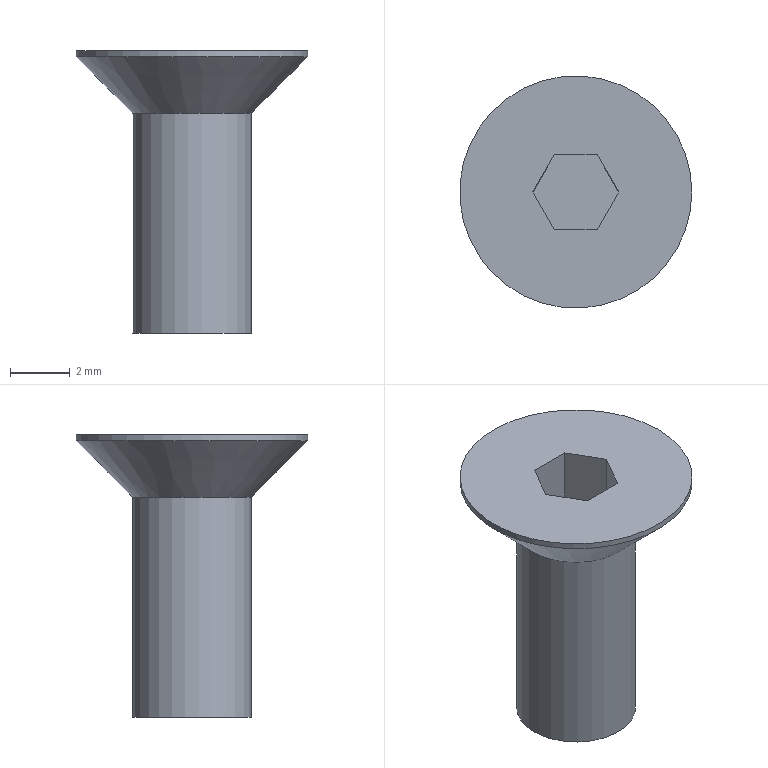Part | STEP file | Tube feed_id378_x_t | 1 solid | 12 faces | box 7.8 x 7.8 x 9.5 mm | volume 142 mm3 | plane 9 | cylinder 2 | cone 1 | commonest cylinder face diameters 4 x1 7.8 x1
STEP:
#1=CARTESIAN_POINT('',(0.,0.,0.));
#2=DIRECTION('',(0.,0.,1.));
#3=DIRECTION('',(1.,0.,0.));
#4=AXIS2_PLACEMENT_3D('',#1,#2,#3);
#5=CARTESIAN_POINT('',(351.278,11.286,-1.5));
#6=VERTEX_POINT('',#5);
#7=CARTESIAN_POINT('',(350.557,10.036,-1.5));
#8=VERTEX_POINT('',#7);
#9=CARTESIAN_POINT('',(351.278,11.286,-1.5));
#10=DIRECTION('',(-0.5,-0.866,0.));
#11=VECTOR('',#10,1.);
#12=LINE('',#9,#11);
#13=CARTESIAN_POINT('',(352.,10.036,-1.5));
#14=DIRECTION('',(0.,0.,1.));
#15=DIRECTION('',(1.,0.,0.));
#16=AXIS2_PLACEMENT_3D('',#13,#14,#15);
#17=PLANE('',#16);
#18=CARTESIAN_POINT('',(-0.7217,1.25));
#19=DIRECTION('',(-0.5,-0.866));
#20=VECTOR('',#19,1.);
#21=LINE('',#18,#20);
#22=(GEOMETRIC_REPRESENTATION_CONTEXT(2)PARAMETRIC_REPRESENTATION_CONTEXT()REPRESENTATION_CONTEXT('',''));
#23=DEFINITIONAL_REPRESENTATION('',(#21),#22);
#24=PCURVE('',#17,#23);
#25=CARTESIAN_POINT('',(351.278,11.286,-4.14));
#26=DIRECTION('',(-0.866,0.5,0.));
#27=DIRECTION('',(-0.5,-0.866,0.));
#28=AXIS2_PLACEMENT_3D('',#25,#26,#27);
#29=PLANE('',#28);
#30=CARTESIAN_POINT('',(0.,2.64));
#31=DIRECTION('',(1.,0.));
#32=VECTOR('',#31,1.);
#33=LINE('',#30,#32);
#34=(GEOMETRIC_REPRESENTATION_CONTEXT(2)PARAMETRIC_REPRESENTATION_CONTEXT()REPRESENTATION_CONTEXT('',''));
#35=DEFINITIONAL_REPRESENTATION('',(#33),#34);
#36=PCURVE('',#29,#35);
#37=SURFACE_CURVE('',#12,(#24,#36),.PCURVE_S1.);
#38=EDGE_CURVE('',#6,#8,#37,.T.);
#39=ORIENTED_EDGE('',*,*,#38,.F.);
#40=CARTESIAN_POINT('',(352.722,11.286,-1.5));
#41=VERTEX_POINT('',#40);
#42=CARTESIAN_POINT('',(352.722,11.286,-1.5));
#43=DIRECTION('',(-1.,0.,0.));
#44=VECTOR('',#43,1.);
#45=LINE('',#42,#44);
#46=CARTESIAN_POINT('',(0.7217,1.25));
#47=DIRECTION('',(-1.,0.));
#48=VECTOR('',#47,1.);
#49=LINE('',#46,#48);
#50=(GEOMETRIC_REPRESENTATION_CONTEXT(2)PARAMETRIC_REPRESENTATION_CONTEXT()REPRESENTATION_CONTEXT('',''));
#51=DEFINITIONAL_REPRESENTATION('',(#49),#50);
#52=PCURVE('',#17,#51);
#53=CARTESIAN_POINT('',(352.722,11.286,-4.14));
#54=DIRECTION('',(0.,1.,0.));
#55=DIRECTION('',(-1.,0.,0.));
#56=AXIS2_PLACEMENT_3D('',#53,#54,#55);
#57=PLANE('',#56);
#58=CARTESIAN_POINT('',(0.,2.64));
#59=DIRECTION('',(1.,0.));
#60=VECTOR('',#59,1.);
#61=LINE('',#58,#60);
#62=(GEOMETRIC_REPRESENTATION_CONTEXT(2)PARAMETRIC_REPRESENTATION_CONTEXT()REPRESENTATION_CONTEXT('',''));
#63=DEFINITIONAL_REPRESENTATION('',(#61),#62);
#64=PCURVE('',#57,#63);
#65=SURFACE_CURVE('',#45,(#52,#64),.PCURVE_S1.);
#66=EDGE_CURVE('',#41,#6,#65,.T.);
#67=ORIENTED_EDGE('',*,*,#66,.F.);
#68=CARTESIAN_POINT('',(353.443,10.036,-1.5));
#69=VERTEX_POINT('',#68);
#70=CARTESIAN_POINT('',(353.443,10.036,-1.5));
#71=DIRECTION('',(-0.5,0.866,0.));
#72=VECTOR('',#71,1.);
#73=LINE('',#70,#72);
#74=CARTESIAN_POINT('',(1.443,0.));
#75=DIRECTION('',(-0.5,0.866));
#76=VECTOR('',#75,1.);
#77=LINE('',#74,#76);
#78=(GEOMETRIC_REPRESENTATION_CONTEXT(2)PARAMETRIC_REPRESENTATION_CONTEXT()REPRESENTATION_CONTEXT('',''));
#79=DEFINITIONAL_REPRESENTATION('',(#77),#78);
#80=PCURVE('',#17,#79);
#81=CARTESIAN_POINT('',(353.443,10.036,-4.14));
#82=DIRECTION('',(0.866,0.5,0.));
#83=DIRECTION('',(-0.5,0.866,0.));
#84=AXIS2_PLACEMENT_3D('',#81,#82,#83);
#85=PLANE('',#84);
#86=CARTESIAN_POINT('',(0.,2.64));
#87=DIRECTION('',(1.,0.));
#88=VECTOR('',#87,1.);
#89=LINE('',#86,#88);
#90=(GEOMETRIC_REPRESENTATION_CONTEXT(2)PARAMETRIC_REPRESENTATION_CONTEXT()REPRESENTATION_CONTEXT('',''));
#91=DEFINITIONAL_REPRESENTATION('',(#89),#90);
#92=PCURVE('',#85,#91);
#93=SURFACE_CURVE('',#73,(#80,#92),.PCURVE_S1.);
#94=EDGE_CURVE('',#69,#41,#93,.T.);
#95=ORIENTED_EDGE('',*,*,#94,.F.);
#96=CARTESIAN_POINT('',(352.722,8.786,-1.5));
#97=VERTEX_POINT('',#96);
#98=CARTESIAN_POINT('',(352.722,8.786,-1.5));
#99=DIRECTION('',(0.5,0.866,0.));
#100=VECTOR('',#99,1.);
#101=LINE('',#98,#100);
#102=CARTESIAN_POINT('',(0.7217,-1.25));
#103=DIRECTION('',(0.5,0.866));
#104=VECTOR('',#103,1.);
#105=LINE('',#102,#104);
#106=(GEOMETRIC_REPRESENTATION_CONTEXT(2)PARAMETRIC_REPRESENTATION_CONTEXT()REPRESENTATION_CONTEXT('',''));
#107=DEFINITIONAL_REPRESENTATION('',(#105),#106);
#108=PCURVE('',#17,#107);
#109=CARTESIAN_POINT('',(352.722,8.786,-4.14));
#110=DIRECTION('',(0.866,-0.5,0.));
#111=DIRECTION('',(0.5,0.866,0.));
#112=AXIS2_PLACEMENT_3D('',#109,#110,#111);
#113=PLANE('',#112);
#114=CARTESIAN_POINT('',(0.,2.64));
#115=DIRECTION('',(1.,0.));
#116=VECTOR('',#115,1.);
#117=LINE('',#114,#116);
#118=(GEOMETRIC_REPRESENTATION_CONTEXT(2)PARAMETRIC_REPRESENTATION_CONTEXT()REPRESENTATION_CONTEXT('',''));
#119=DEFINITIONAL_REPRESENTATION('',(#117),#118);
#120=PCURVE('',#113,#119);
#121=SURFACE_CURVE('',#101,(#108,#120),.PCURVE_S1.);
#122=EDGE_CURVE('',#97,#69,#121,.T.);
#123=ORIENTED_EDGE('',*,*,#122,.F.);
#124=CARTESIAN_POINT('',(351.278,8.786,-1.5));
#125=VERTEX_POINT('',#124);
#126=CARTESIAN_POINT('',(351.278,8.786,-1.5));
#127=DIRECTION('',(1.,0.,0.));
#128=VECTOR('',#127,1.);
#129=LINE('',#126,#128);
#130=CARTESIAN_POINT('',(-0.7217,-1.25));
#131=DIRECTION('',(1.,0.));
#132=VECTOR('',#131,1.);
#133=LINE('',#130,#132);
#134=(GEOMETRIC_REPRESENTATION_CONTEXT(2)PARAMETRIC_REPRESENTATION_CONTEXT()REPRESENTATION_CONTEXT('',''));
#135=DEFINITIONAL_REPRESENTATION('',(#133),#134);
#136=PCURVE('',#17,#135);
#137=CARTESIAN_POINT('',(351.278,8.786,-4.14));
#138=DIRECTION('',(0.,-1.,0.));
#139=DIRECTION('',(1.,0.,0.));
#140=AXIS2_PLACEMENT_3D('',#137,#138,#139);
#141=PLANE('',#140);
#142=CARTESIAN_POINT('',(0.,2.64));
#143=DIRECTION('',(1.,0.));
#144=VECTOR('',#143,1.);
#145=LINE('',#142,#144);
#146=(GEOMETRIC_REPRESENTATION_CONTEXT(2)PARAMETRIC_REPRESENTATION_CONTEXT()REPRESENTATION_CONTEXT('',''));
#147=DEFINITIONAL_REPRESENTATION('',(#145),#146);
#148=PCURVE('',#141,#147);
#149=SURFACE_CURVE('',#129,(#136,#148),.PCURVE_S1.);
#150=EDGE_CURVE('',#125,#97,#149,.T.);
#151=ORIENTED_EDGE('',*,*,#150,.F.);
#152=CARTESIAN_POINT('',(350.557,10.036,-1.5));
#153=DIRECTION('',(0.5,-0.866,0.));
#154=VECTOR('',#153,1.);
#155=LINE('',#152,#154);
#156=CARTESIAN_POINT('',(-1.443,0.));
#157=DIRECTION('',(0.5,-0.866));
#158=VECTOR('',#157,1.);
#159=LINE('',#156,#158);
#160=(GEOMETRIC_REPRESENTATION_CONTEXT(2)PARAMETRIC_REPRESENTATION_CONTEXT()REPRESENTATION_CONTEXT('',''));
#161=DEFINITIONAL_REPRESENTATION('',(#159),#160);
#162=PCURVE('',#17,#161);
#163=CARTESIAN_POINT('',(350.557,10.036,-4.14));
#164=DIRECTION('',(-0.866,-0.5,0.));
#165=DIRECTION('',(0.5,-0.866,0.));
#166=AXIS2_PLACEMENT_3D('',#163,#164,#165);
#167=PLANE('',#166);
#168=CARTESIAN_POINT('',(0.,2.64));
#169=DIRECTION('',(1.,0.));
#170=VECTOR('',#169,1.);
#171=LINE('',#168,#170);
#172=(GEOMETRIC_REPRESENTATION_CONTEXT(2)PARAMETRIC_REPRESENTATION_CONTEXT()REPRESENTATION_CONTEXT('',''));
#173=DEFINITIONAL_REPRESENTATION('',(#171),#172);
#174=PCURVE('',#167,#173);
#175=SURFACE_CURVE('',#155,(#162,#174),.PCURVE_S1.);
#176=EDGE_CURVE('',#8,#125,#175,.T.);
#177=ORIENTED_EDGE('',*,*,#176,.F.);
#178=EDGE_LOOP('',(#39,#67,#95,#123,#151,#177));
#179=FACE_BOUND('',#178,.T.);
#180=CARTESIAN_POINT('',(355.9,10.036,-1.5));
#181=VERTEX_POINT('',#180);
#182=CARTESIAN_POINT('',(352.,10.036,-1.5));
#183=DIRECTION('',(0.,0.,1.));
#184=DIRECTION('',(1.,0.,0.));
#185=AXIS2_PLACEMENT_3D('',#182,#183,#184);
#186=CIRCLE('',#185,3.9);
#187=CARTESIAN_POINT('',(0.,0.));
#188=DIRECTION('',(1.,0.));
#189=AXIS2_PLACEMENT_2D('',#187,#188);
#190=CIRCLE('',#189,3.9);
#191=(GEOMETRIC_REPRESENTATION_CONTEXT(2)PARAMETRIC_REPRESENTATION_CONTEXT()REPRESENTATION_CONTEXT('',''));
#192=DEFINITIONAL_REPRESENTATION('',(#190),#191);
#193=PCURVE('',#17,#192);
#194=CARTESIAN_POINT('',(352.,10.036,-1.));
#195=DIRECTION('',(0.,0.,1.));
#196=DIRECTION('',(1.,0.,0.));
#197=AXIS2_PLACEMENT_3D('',#194,#195,#196);
#198=CYLINDRICAL_SURFACE('',#197,3.9);
#199=CARTESIAN_POINT('',(0.,-0.5));
#200=DIRECTION('',(1.,0.));
#201=VECTOR('',#200,1.);
#202=LINE('',#199,#201);
#203=(GEOMETRIC_REPRESENTATION_CONTEXT(2)PARAMETRIC_REPRESENTATION_CONTEXT()REPRESENTATION_CONTEXT('',''));
#204=DEFINITIONAL_REPRESENTATION('',(#202),#203);
#205=PCURVE('',#198,#204);
#206=SURFACE_CURVE('',#186,(#193,#205),.PCURVE_S1.);
#207=EDGE_CURVE('',#181,#181,#206,.T.);
#208=ORIENTED_EDGE('',*,*,#207,.T.);
#209=EDGE_LOOP('',(#208));
#210=FACE_BOUND('',#209,.T.);
#211=ADVANCED_FACE('',(#179,#210),#17,.T.);
#212=CARTESIAN_POINT('',(354.,10.036,-11.));
#213=VERTEX_POINT('',#212);
#214=CARTESIAN_POINT('',(352.,10.036,-11.));
#215=DIRECTION('',(0.,0.,1.));
#216=DIRECTION('',(1.,0.,0.));
#217=AXIS2_PLACEMENT_3D('',#214,#215,#216);
#218=CIRCLE('',#217,2.);
#219=CARTESIAN_POINT('',(352.,10.036,-11.));
#220=DIRECTION('',(0.,0.,1.));
#221=DIRECTION('',(1.,0.,0.));
#222=AXIS2_PLACEMENT_3D('',#219,#220,#221);
#223=PLANE('',#222);
#224=CARTESIAN_POINT('',(0.,0.));
#225=DIRECTION('',(1.,0.));
#226=AXIS2_PLACEMENT_2D('',#224,#225);
#227=CIRCLE('',#226,2.);
#228=(GEOMETRIC_REPRESENTATION_CONTEXT(2)PARAMETRIC_REPRESENTATION_CONTEXT()REPRESENTATION_CONTEXT('',''));
#229=DEFINITIONAL_REPRESENTATION('',(#227),#228);
#230=PCURVE('',#223,#229);
#231=CARTESIAN_POINT('',(352.,10.036,-1.));
#232=DIRECTION('',(0.,0.,1.));
#233=DIRECTION('',(1.,0.,0.));
#234=AXIS2_PLACEMENT_3D('',#231,#232,#233);
#235=CYLINDRICAL_SURFACE('',#234,2.);
#236=CARTESIAN_POINT('',(0.,-10.));
#237=DIRECTION('',(1.,0.));
#238=VECTOR('',#237,1.);
#239=LINE('',#236,#238);
#240=(GEOMETRIC_REPRESENTATION_CONTEXT(2)PARAMETRIC_REPRESENTATION_CONTEXT()REPRESENTATION_CONTEXT('',''));
#241=DEFINITIONAL_REPRESENTATION('',(#239),#240);
#242=PCURVE('',#235,#241);
#243=SURFACE_CURVE('',#218,(#230,#242),.PCURVE_S1.);
#244=EDGE_CURVE('',#213,#213,#243,.T.);
#245=ORIENTED_EDGE('',*,*,#244,.F.);
#246=EDGE_LOOP('',(#245));
#247=FACE_BOUND('',#246,.T.);
#248=ADVANCED_FACE('',(#247),#223,.F.);
#249=ORIENTED_EDGE('',*,*,#244,.T.);
#250=CARTESIAN_POINT('',(354.,10.036,-3.6));
#251=VERTEX_POINT('',#250);
#252=CARTESIAN_POINT('',(354.,10.036,-11.));
#253=CARTESIAN_POINT('',(354.,10.036,-3.6));
#254=B_SPLINE_CURVE_WITH_KNOTS('',1,(#252,#253),.UNSPECIFIED.,.F.,.F.,(2,2),(-10.,-2.6),.PIECEWISE_BEZIER_KNOTS.);
#255=CARTESIAN_POINT('',(6.283,0.));
#256=DIRECTION('',(0.,1.));
#257=VECTOR('',#256,1.);
#258=LINE('',#255,#257);
#259=(GEOMETRIC_REPRESENTATION_CONTEXT(2)PARAMETRIC_REPRESENTATION_CONTEXT()REPRESENTATION_CONTEXT('',''));
#260=DEFINITIONAL_REPRESENTATION('',(#258),#259);
#261=PCURVE('',#235,#260);
#262=CARTESIAN_POINT('',(0.,0.));
#263=DIRECTION('',(0.,1.));
#264=VECTOR('',#263,1.);
#265=LINE('',#262,#264);
#266=(GEOMETRIC_REPRESENTATION_CONTEXT(2)PARAMETRIC_REPRESENTATION_CONTEXT()REPRESENTATION_CONTEXT('',''));
#267=DEFINITIONAL_REPRESENTATION('',(#265),#266);
#268=PCURVE('',#235,#267);
#269=SEAM_CURVE('',#254,(#261,#268),.PCURVE_S1.);
#270=EDGE_CURVE('',#213,#251,#269,.T.);
#271=ORIENTED_EDGE('',*,*,#270,.T.);
#272=CARTESIAN_POINT('',(352.,10.036,-3.6));
#273=DIRECTION('',(0.,0.,1.));
#274=DIRECTION('',(1.,0.,0.));
#275=AXIS2_PLACEMENT_3D('',#272,#273,#274);
#276=CIRCLE('',#275,2.);
#277=CARTESIAN_POINT('',(0.,-2.6));
#278=DIRECTION('',(1.,0.));
#279=VECTOR('',#278,1.);
#280=LINE('',#277,#279);
#281=(GEOMETRIC_REPRESENTATION_CONTEXT(2)PARAMETRIC_REPRESENTATION_CONTEXT()REPRESENTATION_CONTEXT('',''));
#282=DEFINITIONAL_REPRESENTATION('',(#280),#281);
#283=PCURVE('',#235,#282);
#284=CARTESIAN_POINT('',(352.,10.036,-1.7));
#285=DIRECTION('',(0.,0.,1.));
#286=DIRECTION('',(1.,0.,0.));
#287=AXIS2_PLACEMENT_3D('',#284,#285,#286);
#288=CONICAL_SURFACE('',#287,3.9,0.7854);
#289=CARTESIAN_POINT('',(0.,-1.9));
#290=DIRECTION('',(1.,0.));
#291=VECTOR('',#290,1.);
#292=LINE('',#289,#291);
#293=(GEOMETRIC_REPRESENTATION_CONTEXT(2)PARAMETRIC_REPRESENTATION_CONTEXT()REPRESENTATION_CONTEXT('',''));
#294=DEFINITIONAL_REPRESENTATION('',(#292),#293);
#295=PCURVE('',#288,#294);
#296=SURFACE_CURVE('',#276,(#283,#295),.PCURVE_S1.);
#297=EDGE_CURVE('',#251,#251,#296,.T.);
#298=ORIENTED_EDGE('',*,*,#297,.F.);
#299=ORIENTED_EDGE('',*,*,#270,.F.);
#300=EDGE_LOOP('',(#249,#271,#298,#299));
#301=FACE_BOUND('',#300,.T.);
#302=ADVANCED_FACE('',(#301),#235,.T.);
#303=ORIENTED_EDGE('',*,*,#297,.T.);
#304=CARTESIAN_POINT('',(355.9,10.036,-1.7));
#305=VERTEX_POINT('',#304);
#306=CARTESIAN_POINT('',(354.,10.036,-3.6));
#307=CARTESIAN_POINT('',(355.9,10.036,-1.7));
#308=B_SPLINE_CURVE_WITH_KNOTS('',1,(#306,#307),.UNSPECIFIED.,.F.,.F.,(2,2),(-2.687,0.),.PIECEWISE_BEZIER_KNOTS.);
#309=CARTESIAN_POINT('',(6.283,0.));
#310=DIRECTION('',(0.,1.));
#311=VECTOR('',#310,1.);
#312=LINE('',#309,#311);
#313=(GEOMETRIC_REPRESENTATION_CONTEXT(2)PARAMETRIC_REPRESENTATION_CONTEXT()REPRESENTATION_CONTEXT('',''));
#314=DEFINITIONAL_REPRESENTATION('',(#312),#313);
#315=PCURVE('',#288,#314);
#316=CARTESIAN_POINT('',(0.,0.));
#317=DIRECTION('',(0.,1.));
#318=VECTOR('',#317,1.);
#319=LINE('',#316,#318);
#320=(GEOMETRIC_REPRESENTATION_CONTEXT(2)PARAMETRIC_REPRESENTATION_CONTEXT()REPRESENTATION_CONTEXT('',''));
#321=DEFINITIONAL_REPRESENTATION('',(#319),#320);
#322=PCURVE('',#288,#321);
#323=SEAM_CURVE('',#308,(#315,#322),.PCURVE_S1.);
#324=EDGE_CURVE('',#251,#305,#323,.T.);
#325=ORIENTED_EDGE('',*,*,#324,.T.);
#326=CARTESIAN_POINT('',(352.,10.036,-1.7));
#327=DIRECTION('',(0.,0.,1.));
#328=DIRECTION('',(1.,0.,0.));
#329=AXIS2_PLACEMENT_3D('',#326,#327,#328);
#330=CIRCLE('',#329,3.9);
#331=CARTESIAN_POINT('',(0.,0.));
#332=DIRECTION('',(1.,0.));
#333=VECTOR('',#332,1.);
#334=LINE('',#331,#333);
#335=(GEOMETRIC_REPRESENTATION_CONTEXT(2)PARAMETRIC_REPRESENTATION_CONTEXT()REPRESENTATION_CONTEXT('',''));
#336=DEFINITIONAL_REPRESENTATION('',(#334),#335);
#337=PCURVE('',#288,#336);
#338=CARTESIAN_POINT('',(0.,-0.7));
#339=DIRECTION('',(1.,0.));
#340=VECTOR('',#339,1.);
#341=LINE('',#338,#340);
#342=(GEOMETRIC_REPRESENTATION_CONTEXT(2)PARAMETRIC_REPRESENTATION_CONTEXT()REPRESENTATION_CONTEXT('',''));
#343=DEFINITIONAL_REPRESENTATION('',(#341),#342);
#344=PCURVE('',#198,#343);
#345=SURFACE_CURVE('',#330,(#337,#344),.PCURVE_S1.);
#346=EDGE_CURVE('',#305,#305,#345,.T.);
#347=ORIENTED_EDGE('',*,*,#346,.F.);
#348=ORIENTED_EDGE('',*,*,#324,.F.);
#349=EDGE_LOOP('',(#303,#325,#347,#348));
#350=FACE_BOUND('',#349,.T.);
#351=ADVANCED_FACE('',(#350),#288,.T.);
#352=ORIENTED_EDGE('',*,*,#346,.T.);
#353=CARTESIAN_POINT('',(355.9,10.036,-1.7));
#354=CARTESIAN_POINT('',(355.9,10.036,-1.5));
#355=B_SPLINE_CURVE_WITH_KNOTS('',1,(#353,#354),.UNSPECIFIED.,.F.,.F.,(2,2),(-0.7,-0.5),.PIECEWISE_BEZIER_KNOTS.);
#356=CARTESIAN_POINT('',(6.283,0.));
#357=DIRECTION('',(0.,1.));
#358=VECTOR('',#357,1.);
#359=LINE('',#356,#358);
#360=(GEOMETRIC_REPRESENTATION_CONTEXT(2)PARAMETRIC_REPRESENTATION_CONTEXT()REPRESENTATION_CONTEXT('',''));
#361=DEFINITIONAL_REPRESENTATION('',(#359),#360);
#362=PCURVE('',#198,#361);
#363=CARTESIAN_POINT('',(0.,0.));
#364=DIRECTION('',(0.,1.));
#365=VECTOR('',#364,1.);
#366=LINE('',#363,#365);
#367=(GEOMETRIC_REPRESENTATION_CONTEXT(2)PARAMETRIC_REPRESENTATION_CONTEXT()REPRESENTATION_CONTEXT('',''));
#368=DEFINITIONAL_REPRESENTATION('',(#366),#367);
#369=PCURVE('',#198,#368);
#370=SEAM_CURVE('',#355,(#362,#369),.PCURVE_S1.);
#371=EDGE_CURVE('',#305,#181,#370,.T.);
#372=ORIENTED_EDGE('',*,*,#371,.T.);
#373=ORIENTED_EDGE('',*,*,#207,.F.);
#374=ORIENTED_EDGE('',*,*,#371,.F.);
#375=EDGE_LOOP('',(#352,#372,#373,#374));
#376=FACE_BOUND('',#375,.T.);
#377=ADVANCED_FACE('',(#376),#198,.T.);
#378=ORIENTED_EDGE('',*,*,#38,.T.);
#379=CARTESIAN_POINT('',(350.557,10.036,-4.14));
#380=VERTEX_POINT('',#379);
#381=CARTESIAN_POINT('',(350.557,10.036,-4.14));
#382=DIRECTION('',(0.,0.,-1.));
#383=VECTOR('',#382,1.);
#384=LINE('',#381,#383);
#385=CARTESIAN_POINT('',(1.443,0.));
#386=DIRECTION('',(0.,-1.));
#387=VECTOR('',#386,1.);
#388=LINE('',#385,#387);
#389=(GEOMETRIC_REPRESENTATION_CONTEXT(2)PARAMETRIC_REPRESENTATION_CONTEXT()REPRESENTATION_CONTEXT('',''));
#390=DEFINITIONAL_REPRESENTATION('',(#388),#389);
#391=PCURVE('',#29,#390);
#392=CARTESIAN_POINT('',(0.,0.));
#393=DIRECTION('',(0.,-1.));
#394=VECTOR('',#393,1.);
#395=LINE('',#392,#394);
#396=(GEOMETRIC_REPRESENTATION_CONTEXT(2)PARAMETRIC_REPRESENTATION_CONTEXT()REPRESENTATION_CONTEXT('',''));
#397=DEFINITIONAL_REPRESENTATION('',(#395),#396);
#398=PCURVE('',#167,#397);
#399=SURFACE_CURVE('',#384,(#391,#398),.PCURVE_S1.);
#400=EDGE_CURVE('',#8,#380,#399,.T.);
#401=ORIENTED_EDGE('',*,*,#400,.T.);
#402=CARTESIAN_POINT('',(351.278,11.286,-4.14));
#403=VERTEX_POINT('',#402);
#404=CARTESIAN_POINT('',(351.278,11.286,-4.14));
#405=DIRECTION('',(0.5,0.866,0.));
#406=VECTOR('',#405,1.);
#407=LINE('',#404,#406);
#408=CARTESIAN_POINT('',(0.,0.));
#409=DIRECTION('',(-1.,0.));
#410=VECTOR('',#409,1.);
#411=LINE('',#408,#410);
#412=(GEOMETRIC_REPRESENTATION_CONTEXT(2)PARAMETRIC_REPRESENTATION_CONTEXT()REPRESENTATION_CONTEXT('',''));
#413=DEFINITIONAL_REPRESENTATION('',(#411),#412);
#414=PCURVE('',#29,#413);
#415=CARTESIAN_POINT('',(352.,10.036,-4.14));
#416=DIRECTION('',(0.,0.,1.));
#417=DIRECTION('',(1.,0.,0.));
#418=AXIS2_PLACEMENT_3D('',#415,#416,#417);
#419=PLANE('',#418);
#420=CARTESIAN_POINT('',(-0.7217,1.25));
#421=DIRECTION('',(0.5,0.866));
#422=VECTOR('',#421,1.);
#423=LINE('',#420,#422);
#424=(GEOMETRIC_REPRESENTATION_CONTEXT(2)PARAMETRIC_REPRESENTATION_CONTEXT()REPRESENTATION_CONTEXT('',''));
#425=DEFINITIONAL_REPRESENTATION('',(#423),#424);
#426=PCURVE('',#419,#425);
#427=SURFACE_CURVE('',#407,(#414,#426),.PCURVE_S1.);
#428=EDGE_CURVE('',#380,#403,#427,.T.);
#429=ORIENTED_EDGE('',*,*,#428,.T.);
#430=CARTESIAN_POINT('',(351.278,11.286,-4.14));
#431=DIRECTION('',(0.,0.,-1.));
#432=VECTOR('',#431,1.);
#433=LINE('',#430,#432);
#434=CARTESIAN_POINT('',(0.,0.));
#435=DIRECTION('',(0.,-1.));
#436=VECTOR('',#435,1.);
#437=LINE('',#434,#436);
#438=(GEOMETRIC_REPRESENTATION_CONTEXT(2)PARAMETRIC_REPRESENTATION_CONTEXT()REPRESENTATION_CONTEXT('',''));
#439=DEFINITIONAL_REPRESENTATION('',(#437),#438);
#440=PCURVE('',#29,#439);
#441=CARTESIAN_POINT('',(1.443,0.));
#442=DIRECTION('',(0.,-1.));
#443=VECTOR('',#442,1.);
#444=LINE('',#441,#443);
#445=(GEOMETRIC_REPRESENTATION_CONTEXT(2)PARAMETRIC_REPRESENTATION_CONTEXT()REPRESENTATION_CONTEXT('',''));
#446=DEFINITIONAL_REPRESENTATION('',(#444),#445);
#447=PCURVE('',#57,#446);
#448=SURFACE_CURVE('',#433,(#440,#447),.PCURVE_S1.);
#449=EDGE_CURVE('',#6,#403,#448,.T.);
#450=ORIENTED_EDGE('',*,*,#449,.F.);
#451=EDGE_LOOP('',(#378,#401,#429,#450));
#452=FACE_BOUND('',#451,.T.);
#453=ADVANCED_FACE('',(#452),#29,.F.);
#454=ORIENTED_EDGE('',*,*,#176,.T.);
#455=CARTESIAN_POINT('',(351.278,8.786,-4.14));
#456=VERTEX_POINT('',#455);
#457=CARTESIAN_POINT('',(351.278,8.786,-4.14));
#458=DIRECTION('',(0.,0.,-1.));
#459=VECTOR('',#458,1.);
#460=LINE('',#457,#459);
#461=CARTESIAN_POINT('',(1.443,0.));
#462=DIRECTION('',(0.,-1.));
#463=VECTOR('',#462,1.);
#464=LINE('',#461,#463);
#465=(GEOMETRIC_REPRESENTATION_CONTEXT(2)PARAMETRIC_REPRESENTATION_CONTEXT()REPRESENTATION_CONTEXT('',''));
#466=DEFINITIONAL_REPRESENTATION('',(#464),#465);
#467=PCURVE('',#167,#466);
#468=CARTESIAN_POINT('',(0.,0.));
#469=DIRECTION('',(0.,-1.));
#470=VECTOR('',#469,1.);
#471=LINE('',#468,#470);
#472=(GEOMETRIC_REPRESENTATION_CONTEXT(2)PARAMETRIC_REPRESENTATION_CONTEXT()REPRESENTATION_CONTEXT('',''));
#473=DEFINITIONAL_REPRESENTATION('',(#471),#472);
#474=PCURVE('',#141,#473);
#475=SURFACE_CURVE('',#460,(#467,#474),.PCURVE_S1.);
#476=EDGE_CURVE('',#125,#456,#475,.T.);
#477=ORIENTED_EDGE('',*,*,#476,.T.);
#478=CARTESIAN_POINT('',(350.557,10.036,-4.14));
#479=DIRECTION('',(-0.5,0.866,0.));
#480=VECTOR('',#479,1.);
#481=LINE('',#478,#480);
#482=CARTESIAN_POINT('',(0.,0.));
#483=DIRECTION('',(-1.,0.));
#484=VECTOR('',#483,1.);
#485=LINE('',#482,#484);
#486=(GEOMETRIC_REPRESENTATION_CONTEXT(2)PARAMETRIC_REPRESENTATION_CONTEXT()REPRESENTATION_CONTEXT('',''));
#487=DEFINITIONAL_REPRESENTATION('',(#485),#486);
#488=PCURVE('',#167,#487);
#489=CARTESIAN_POINT('',(-1.443,0.));
#490=DIRECTION('',(-0.5,0.866));
#491=VECTOR('',#490,1.);
#492=LINE('',#489,#491);
#493=(GEOMETRIC_REPRESENTATION_CONTEXT(2)PARAMETRIC_REPRESENTATION_CONTEXT()REPRESENTATION_CONTEXT('',''));
#494=DEFINITIONAL_REPRESENTATION('',(#492),#493);
#495=PCURVE('',#419,#494);
#496=SURFACE_CURVE('',#481,(#488,#495),.PCURVE_S1.);
#497=EDGE_CURVE('',#456,#380,#496,.T.);
#498=ORIENTED_EDGE('',*,*,#497,.T.);
#499=ORIENTED_EDGE('',*,*,#400,.F.);
#500=EDGE_LOOP('',(#454,#477,#498,#499));
#501=FACE_BOUND('',#500,.T.);
#502=ADVANCED_FACE('',(#501),#167,.F.);
#503=ORIENTED_EDGE('',*,*,#150,.T.);
#504=CARTESIAN_POINT('',(352.722,8.786,-4.14));
#505=VERTEX_POINT('',#504);
#506=CARTESIAN_POINT('',(352.722,8.786,-4.14));
#507=DIRECTION('',(0.,0.,-1.));
#508=VECTOR('',#507,1.);
#509=LINE('',#506,#508);
#510=CARTESIAN_POINT('',(1.443,0.));
#511=DIRECTION('',(0.,-1.));
#512=VECTOR('',#511,1.);
#513=LINE('',#510,#512);
#514=(GEOMETRIC_REPRESENTATION_CONTEXT(2)PARAMETRIC_REPRESENTATION_CONTEXT()REPRESENTATION_CONTEXT('',''));
#515=DEFINITIONAL_REPRESENTATION('',(#513),#514);
#516=PCURVE('',#141,#515);
#517=CARTESIAN_POINT('',(0.,0.));
#518=DIRECTION('',(0.,-1.));
#519=VECTOR('',#518,1.);
#520=LINE('',#517,#519);
#521=(GEOMETRIC_REPRESENTATION_CONTEXT(2)PARAMETRIC_REPRESENTATION_CONTEXT()REPRESENTATION_CONTEXT('',''));
#522=DEFINITIONAL_REPRESENTATION('',(#520),#521);
#523=PCURVE('',#113,#522);
#524=SURFACE_CURVE('',#509,(#516,#523),.PCURVE_S1.);
#525=EDGE_CURVE('',#97,#505,#524,.T.);
#526=ORIENTED_EDGE('',*,*,#525,.T.);
#527=CARTESIAN_POINT('',(351.278,8.786,-4.14));
#528=DIRECTION('',(-1.,0.,0.));
#529=VECTOR('',#528,1.);
#530=LINE('',#527,#529);
#531=CARTESIAN_POINT('',(0.,0.));
#532=DIRECTION('',(-1.,0.));
#533=VECTOR('',#532,1.);
#534=LINE('',#531,#533);
#535=(GEOMETRIC_REPRESENTATION_CONTEXT(2)PARAMETRIC_REPRESENTATION_CONTEXT()REPRESENTATION_CONTEXT('',''));
#536=DEFINITIONAL_REPRESENTATION('',(#534),#535);
#537=PCURVE('',#141,#536);
#538=CARTESIAN_POINT('',(-0.7217,-1.25));
#539=DIRECTION('',(-1.,0.));
#540=VECTOR('',#539,1.);
#541=LINE('',#538,#540);
#542=(GEOMETRIC_REPRESENTATION_CONTEXT(2)PARAMETRIC_REPRESENTATION_CONTEXT()REPRESENTATION_CONTEXT('',''));
#543=DEFINITIONAL_REPRESENTATION('',(#541),#542);
#544=PCURVE('',#419,#543);
#545=SURFACE_CURVE('',#530,(#537,#544),.PCURVE_S1.);
#546=EDGE_CURVE('',#505,#456,#545,.T.);
#547=ORIENTED_EDGE('',*,*,#546,.T.);
#548=ORIENTED_EDGE('',*,*,#476,.F.);
#549=EDGE_LOOP('',(#503,#526,#547,#548));
#550=FACE_BOUND('',#549,.T.);
#551=ADVANCED_FACE('',(#550),#141,.F.);
#552=ORIENTED_EDGE('',*,*,#122,.T.);
#553=CARTESIAN_POINT('',(353.443,10.036,-4.14));
#554=VERTEX_POINT('',#553);
#555=CARTESIAN_POINT('',(353.443,10.036,-4.14));
#556=DIRECTION('',(0.,0.,-1.));
#557=VECTOR('',#556,1.);
#558=LINE('',#555,#557);
#559=CARTESIAN_POINT('',(1.443,0.));
#560=DIRECTION('',(0.,-1.));
#561=VECTOR('',#560,1.);
#562=LINE('',#559,#561);
#563=(GEOMETRIC_REPRESENTATION_CONTEXT(2)PARAMETRIC_REPRESENTATION_CONTEXT()REPRESENTATION_CONTEXT('',''));
#564=DEFINITIONAL_REPRESENTATION('',(#562),#563);
#565=PCURVE('',#113,#564);
#566=CARTESIAN_POINT('',(0.,0.));
#567=DIRECTION('',(0.,-1.));
#568=VECTOR('',#567,1.);
#569=LINE('',#566,#568);
#570=(GEOMETRIC_REPRESENTATION_CONTEXT(2)PARAMETRIC_REPRESENTATION_CONTEXT()REPRESENTATION_CONTEXT('',''));
#571=DEFINITIONAL_REPRESENTATION('',(#569),#570);
#572=PCURVE('',#85,#571);
#573=SURFACE_CURVE('',#558,(#565,#572),.PCURVE_S1.);
#574=EDGE_CURVE('',#69,#554,#573,.T.);
#575=ORIENTED_EDGE('',*,*,#574,.T.);
#576=CARTESIAN_POINT('',(352.722,8.786,-4.14));
#577=DIRECTION('',(-0.5,-0.866,0.));
#578=VECTOR('',#577,1.);
#579=LINE('',#576,#578);
#580=CARTESIAN_POINT('',(0.,0.));
#581=DIRECTION('',(-1.,0.));
#582=VECTOR('',#581,1.);
#583=LINE('',#580,#582);
#584=(GEOMETRIC_REPRESENTATION_CONTEXT(2)PARAMETRIC_REPRESENTATION_CONTEXT()REPRESENTATION_CONTEXT('',''));
#585=DEFINITIONAL_REPRESENTATION('',(#583),#584);
#586=PCURVE('',#113,#585);
#587=CARTESIAN_POINT('',(0.7217,-1.25));
#588=DIRECTION('',(-0.5,-0.866));
#589=VECTOR('',#588,1.);
#590=LINE('',#587,#589);
#591=(GEOMETRIC_REPRESENTATION_CONTEXT(2)PARAMETRIC_REPRESENTATION_CONTEXT()REPRESENTATION_CONTEXT('',''));
#592=DEFINITIONAL_REPRESENTATION('',(#590),#591);
#593=PCURVE('',#419,#592);
#594=SURFACE_CURVE('',#579,(#586,#593),.PCURVE_S1.);
#595=EDGE_CURVE('',#554,#505,#594,.T.);
#596=ORIENTED_EDGE('',*,*,#595,.T.);
#597=ORIENTED_EDGE('',*,*,#525,.F.);
#598=EDGE_LOOP('',(#552,#575,#596,#597));
#599=FACE_BOUND('',#598,.T.);
#600=ADVANCED_FACE('',(#599),#113,.F.);
#601=ORIENTED_EDGE('',*,*,#94,.T.);
#602=CARTESIAN_POINT('',(352.722,11.286,-4.14));
#603=VERTEX_POINT('',#602);
#604=CARTESIAN_POINT('',(352.722,11.286,-4.14));
#605=DIRECTION('',(0.,0.,-1.));
#606=VECTOR('',#605,1.);
#607=LINE('',#604,#606);
#608=CARTESIAN_POINT('',(1.443,0.));
#609=DIRECTION('',(0.,-1.));
#610=VECTOR('',#609,1.);
#611=LINE('',#608,#610);
#612=(GEOMETRIC_REPRESENTATION_CONTEXT(2)PARAMETRIC_REPRESENTATION_CONTEXT()REPRESENTATION_CONTEXT('',''));
#613=DEFINITIONAL_REPRESENTATION('',(#611),#612);
#614=PCURVE('',#85,#613);
#615=CARTESIAN_POINT('',(0.,0.));
#616=DIRECTION('',(0.,-1.));
#617=VECTOR('',#616,1.);
#618=LINE('',#615,#617);
#619=(GEOMETRIC_REPRESENTATION_CONTEXT(2)PARAMETRIC_REPRESENTATION_CONTEXT()REPRESENTATION_CONTEXT('',''));
#620=DEFINITIONAL_REPRESENTATION('',(#618),#619);
#621=PCURVE('',#57,#620);
#622=SURFACE_CURVE('',#607,(#614,#621),.PCURVE_S1.);
#623=EDGE_CURVE('',#41,#603,#622,.T.);
#624=ORIENTED_EDGE('',*,*,#623,.T.);
#625=CARTESIAN_POINT('',(353.443,10.036,-4.14));
#626=DIRECTION('',(0.5,-0.866,0.));
#627=VECTOR('',#626,1.);
#628=LINE('',#625,#627);
#629=CARTESIAN_POINT('',(0.,0.));
#630=DIRECTION('',(-1.,0.));
#631=VECTOR('',#630,1.);
#632=LINE('',#629,#631);
#633=(GEOMETRIC_REPRESENTATION_CONTEXT(2)PARAMETRIC_REPRESENTATION_CONTEXT()REPRESENTATION_CONTEXT('',''));
#634=DEFINITIONAL_REPRESENTATION('',(#632),#633);
#635=PCURVE('',#85,#634);
#636=CARTESIAN_POINT('',(1.443,0.));
#637=DIRECTION('',(0.5,-0.866));
#638=VECTOR('',#637,1.);
#639=LINE('',#636,#638);
#640=(GEOMETRIC_REPRESENTATION_CONTEXT(2)PARAMETRIC_REPRESENTATION_CONTEXT()REPRESENTATION_CONTEXT('',''));
#641=DEFINITIONAL_REPRESENTATION('',(#639),#640);
#642=PCURVE('',#419,#641);
#643=SURFACE_CURVE('',#628,(#635,#642),.PCURVE_S1.);
#644=EDGE_CURVE('',#603,#554,#643,.T.);
#645=ORIENTED_EDGE('',*,*,#644,.T.);
#646=ORIENTED_EDGE('',*,*,#574,.F.);
#647=EDGE_LOOP('',(#601,#624,#645,#646));
#648=FACE_BOUND('',#647,.T.);
#649=ADVANCED_FACE('',(#648),#85,.F.);
#650=ORIENTED_EDGE('',*,*,#66,.T.);
#651=ORIENTED_EDGE('',*,*,#449,.T.);
#652=CARTESIAN_POINT('',(352.722,11.286,-4.14));
#653=DIRECTION('',(1.,0.,0.));
#654=VECTOR('',#653,1.);
#655=LINE('',#652,#654);
#656=CARTESIAN_POINT('',(0.,0.));
#657=DIRECTION('',(-1.,0.));
#658=VECTOR('',#657,1.);
#659=LINE('',#656,#658);
#660=(GEOMETRIC_REPRESENTATION_CONTEXT(2)PARAMETRIC_REPRESENTATION_CONTEXT()REPRESENTATION_CONTEXT('',''));
#661=DEFINITIONAL_REPRESENTATION('',(#659),#660);
#662=PCURVE('',#57,#661);
#663=CARTESIAN_POINT('',(0.7217,1.25));
#664=DIRECTION('',(1.,0.));
#665=VECTOR('',#664,1.);
#666=LINE('',#663,#665);
#667=(GEOMETRIC_REPRESENTATION_CONTEXT(2)PARAMETRIC_REPRESENTATION_CONTEXT()REPRESENTATION_CONTEXT('',''));
#668=DEFINITIONAL_REPRESENTATION('',(#666),#667);
#669=PCURVE('',#419,#668);
#670=SURFACE_CURVE('',#655,(#662,#669),.PCURVE_S1.);
#671=EDGE_CURVE('',#403,#603,#670,.T.);
#672=ORIENTED_EDGE('',*,*,#671,.T.);
#673=ORIENTED_EDGE('',*,*,#623,.F.);
#674=EDGE_LOOP('',(#650,#651,#672,#673));
#675=FACE_BOUND('',#674,.T.);
#676=ADVANCED_FACE('',(#675),#57,.F.);
#677=ORIENTED_EDGE('',*,*,#428,.F.);
#678=ORIENTED_EDGE('',*,*,#497,.F.);
#679=ORIENTED_EDGE('',*,*,#546,.F.);
#680=ORIENTED_EDGE('',*,*,#595,.F.);
#681=ORIENTED_EDGE('',*,*,#644,.F.);
#682=ORIENTED_EDGE('',*,*,#671,.F.);
#683=EDGE_LOOP('',(#677,#678,#679,#680,#681,#682));
#684=FACE_BOUND('',#683,.T.);
#685=ADVANCED_FACE('',(#684),#419,.T.);
#686=CLOSED_SHELL('',(#211,#248,#302,#351,#377,#453,#502,#551,#600,#649,#676,#685));
#687=MANIFOLD_SOLID_BREP('',#686);
#688=(LENGTH_UNIT()NAMED_UNIT(*)SI_UNIT(.MILLI.,.METRE.));
#689=UNCERTAINTY_MEASURE_WITH_UNIT(LENGTH_MEASURE(0.000002),#688,'','');
#690=(NAMED_UNIT(*)PLANE_ANGLE_UNIT()SI_UNIT($,.RADIAN.));
#691=(NAMED_UNIT(*)SI_UNIT($,.STERADIAN.)SOLID_ANGLE_UNIT());
#692=(GEOMETRIC_REPRESENTATION_CONTEXT(3)GLOBAL_UNCERTAINTY_ASSIGNED_CONTEXT((#689))GLOBAL_UNIT_ASSIGNED_CONTEXT((#688,#690,#691))REPRESENTATION_CONTEXT('',''));
#693=ADVANCED_BREP_SHAPE_REPRESENTATION('',(#4,#687),#692);